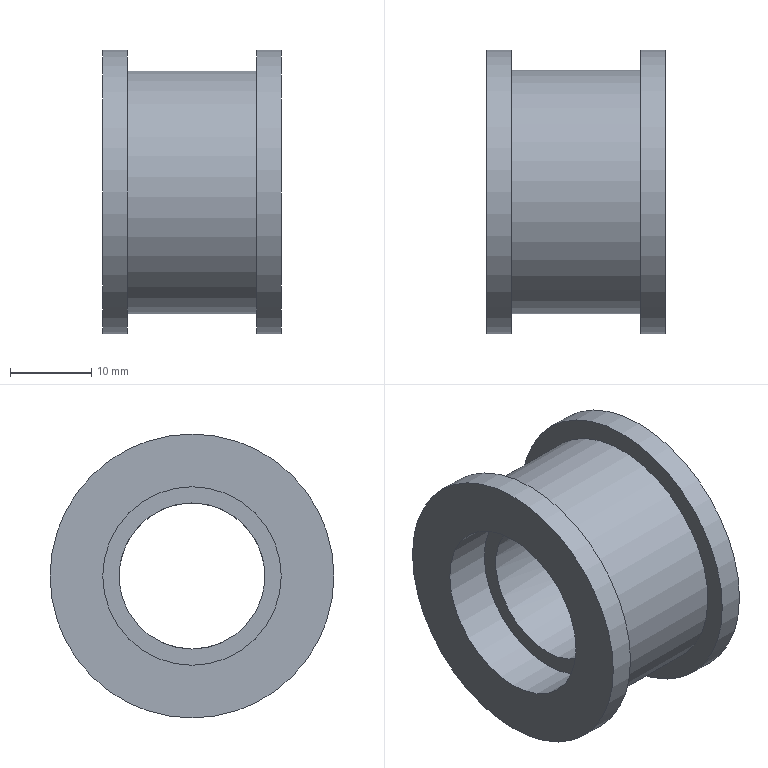Part | NX | 1 solid | 12 faces | box 22 x 35 x 35 mm | volume 9976 mm3 | plane 6 | cylinder 6 | commonest cylinder face diameters 22 x2 35 x2 18 x1 30 x1
STEP:
#1=CARTESIAN_POINT('',(-11.,0.,-17.5));
#2=VERTEX_POINT('',#1);
#3=CARTESIAN_POINT('',(-11.,0.,0.));
#4=DIRECTION('',(1.,0.,0.));
#5=DIRECTION('',(0.,0.,-1.));
#6=AXIS2_PLACEMENT_3D('',#3,#4,#5);
#7=CIRCLE('',#6,17.5);
#8=EDGE_CURVE('',#2,#2,#7,.T.);
#9=ORIENTED_EDGE('',*,*,#8,.F.);
#10=EDGE_LOOP('',(#9));
#11=FACE_BOUND('',#10,.T.);
#12=CARTESIAN_POINT('',(-11.,0.,-11.));
#13=VERTEX_POINT('',#12);
#14=CARTESIAN_POINT('',(-11.,0.,0.));
#15=DIRECTION('',(1.,0.,0.));
#16=DIRECTION('',(0.,0.,-1.));
#17=AXIS2_PLACEMENT_3D('',#14,#15,#16);
#18=CIRCLE('',#17,11.);
#19=EDGE_CURVE('',#13,#13,#18,.T.);
#20=ORIENTED_EDGE('',*,*,#19,.T.);
#21=EDGE_LOOP('',(#20));
#22=FACE_BOUND('',#21,.T.);
#23=CARTESIAN_POINT('',(-11.,0.,0.));
#24=DIRECTION('',(1.,0.,0.));
#25=DIRECTION('',(0.,0.,-1.));
#26=AXIS2_PLACEMENT_3D('',#23,#24,#25);
#27=PLANE('',#26);
#28=ADVANCED_FACE('',(#11,#22),#27,.F.);
#29=ORIENTED_EDGE('',*,*,#8,.T.);
#30=EDGE_LOOP('',(#29));
#31=FACE_BOUND('',#30,.T.);
#32=CARTESIAN_POINT('',(-8.,0.,-17.5));
#33=VERTEX_POINT('',#32);
#34=CARTESIAN_POINT('',(-8.,0.,0.));
#35=DIRECTION('',(1.,0.,0.));
#36=DIRECTION('',(0.,0.,-1.));
#37=AXIS2_PLACEMENT_3D('',#34,#35,#36);
#38=CIRCLE('',#37,17.5);
#39=EDGE_CURVE('',#33,#33,#38,.T.);
#40=ORIENTED_EDGE('',*,*,#39,.F.);
#41=EDGE_LOOP('',(#40));
#42=FACE_BOUND('',#41,.T.);
#43=CARTESIAN_POINT('',(11.,0.,0.));
#44=DIRECTION('',(-1.,0.,0.));
#45=DIRECTION('',(0.,0.,1.));
#46=AXIS2_PLACEMENT_3D('',#43,#44,#45);
#47=CYLINDRICAL_SURFACE('',#46,17.5);
#48=ADVANCED_FACE('',(#31,#42),#47,.T.);
#49=CARTESIAN_POINT('',(-8.,0.,-15.));
#50=VERTEX_POINT('',#49);
#51=CARTESIAN_POINT('',(-8.,0.,0.));
#52=DIRECTION('',(1.,0.,0.));
#53=DIRECTION('',(0.,0.,-1.));
#54=AXIS2_PLACEMENT_3D('',#51,#52,#53);
#55=CIRCLE('',#54,15.);
#56=EDGE_CURVE('',#50,#50,#55,.T.);
#57=ORIENTED_EDGE('',*,*,#56,.F.);
#58=EDGE_LOOP('',(#57));
#59=FACE_BOUND('',#58,.T.);
#60=ORIENTED_EDGE('',*,*,#39,.T.);
#61=EDGE_LOOP('',(#60));
#62=FACE_BOUND('',#61,.T.);
#63=CARTESIAN_POINT('',(-8.,0.,0.));
#64=DIRECTION('',(1.,0.,0.));
#65=DIRECTION('',(0.,0.,-1.));
#66=AXIS2_PLACEMENT_3D('',#63,#64,#65);
#67=PLANE('',#66);
#68=ADVANCED_FACE('',(#59,#62),#67,.T.);
#69=CARTESIAN_POINT('',(8.,0.,-15.));
#70=VERTEX_POINT('',#69);
#71=CARTESIAN_POINT('',(8.,0.,0.));
#72=DIRECTION('',(1.,0.,0.));
#73=DIRECTION('',(0.,0.,-1.));
#74=AXIS2_PLACEMENT_3D('',#71,#72,#73);
#75=CIRCLE('',#74,15.);
#76=EDGE_CURVE('',#70,#70,#75,.T.);
#77=ORIENTED_EDGE('',*,*,#76,.T.);
#78=EDGE_LOOP('',(#77));
#79=FACE_BOUND('',#78,.T.);
#80=CARTESIAN_POINT('',(8.,0.,-17.5));
#81=VERTEX_POINT('',#80);
#82=CARTESIAN_POINT('',(8.,0.,0.));
#83=DIRECTION('',(1.,0.,0.));
#84=DIRECTION('',(0.,0.,-1.));
#85=AXIS2_PLACEMENT_3D('',#82,#83,#84);
#86=CIRCLE('',#85,17.5);
#87=EDGE_CURVE('',#81,#81,#86,.T.);
#88=ORIENTED_EDGE('',*,*,#87,.F.);
#89=EDGE_LOOP('',(#88));
#90=FACE_BOUND('',#89,.T.);
#91=CARTESIAN_POINT('',(8.,0.,0.));
#92=DIRECTION('',(1.,0.,0.));
#93=DIRECTION('',(0.,0.,-1.));
#94=AXIS2_PLACEMENT_3D('',#91,#92,#93);
#95=PLANE('',#94);
#96=ADVANCED_FACE('',(#79,#90),#95,.F.);
#97=ORIENTED_EDGE('',*,*,#56,.T.);
#98=EDGE_LOOP('',(#97));
#99=FACE_BOUND('',#98,.T.);
#100=ORIENTED_EDGE('',*,*,#76,.F.);
#101=EDGE_LOOP('',(#100));
#102=FACE_BOUND('',#101,.T.);
#103=CARTESIAN_POINT('',(-8.,0.,0.));
#104=DIRECTION('',(1.,0.,0.));
#105=DIRECTION('',(0.,0.,-1.));
#106=AXIS2_PLACEMENT_3D('',#103,#104,#105);
#107=CYLINDRICAL_SURFACE('',#106,15.);
#108=ADVANCED_FACE('',(#99,#102),#107,.T.);
#109=CARTESIAN_POINT('',(11.,0.,-11.));
#110=VERTEX_POINT('',#109);
#111=CARTESIAN_POINT('',(11.,0.,0.));
#112=DIRECTION('',(1.,0.,0.));
#113=DIRECTION('',(0.,0.,-1.));
#114=AXIS2_PLACEMENT_3D('',#111,#112,#113);
#115=CIRCLE('',#114,11.);
#116=EDGE_CURVE('',#110,#110,#115,.T.);
#117=ORIENTED_EDGE('',*,*,#116,.F.);
#118=EDGE_LOOP('',(#117));
#119=FACE_BOUND('',#118,.T.);
#120=CARTESIAN_POINT('',(11.,0.,-17.5));
#121=VERTEX_POINT('',#120);
#122=CARTESIAN_POINT('',(11.,0.,0.));
#123=DIRECTION('',(1.,0.,0.));
#124=DIRECTION('',(0.,0.,-1.));
#125=AXIS2_PLACEMENT_3D('',#122,#123,#124);
#126=CIRCLE('',#125,17.5);
#127=EDGE_CURVE('',#121,#121,#126,.T.);
#128=ORIENTED_EDGE('',*,*,#127,.T.);
#129=EDGE_LOOP('',(#128));
#130=FACE_BOUND('',#129,.T.);
#131=CARTESIAN_POINT('',(11.,0.,0.));
#132=DIRECTION('',(1.,0.,0.));
#133=DIRECTION('',(0.,0.,-1.));
#134=AXIS2_PLACEMENT_3D('',#131,#132,#133);
#135=PLANE('',#134);
#136=ADVANCED_FACE('',(#119,#130),#135,.T.);
#137=ORIENTED_EDGE('',*,*,#87,.T.);
#138=EDGE_LOOP('',(#137));
#139=FACE_BOUND('',#138,.T.);
#140=ORIENTED_EDGE('',*,*,#127,.F.);
#141=EDGE_LOOP('',(#140));
#142=FACE_BOUND('',#141,.T.);
#143=CARTESIAN_POINT('',(11.,0.,0.));
#144=DIRECTION('',(-1.,0.,0.));
#145=DIRECTION('',(0.,0.,1.));
#146=AXIS2_PLACEMENT_3D('',#143,#144,#145);
#147=CYLINDRICAL_SURFACE('',#146,17.5);
#148=ADVANCED_FACE('',(#139,#142),#147,.T.);
#149=CARTESIAN_POINT('',(5.,0.,-11.));
#150=VERTEX_POINT('',#149);
#151=CARTESIAN_POINT('',(5.,0.,0.));
#152=DIRECTION('',(1.,0.,0.));
#153=DIRECTION('',(0.,0.,-1.));
#154=AXIS2_PLACEMENT_3D('',#151,#152,#153);
#155=CIRCLE('',#154,11.);
#156=EDGE_CURVE('',#150,#150,#155,.T.);
#157=ORIENTED_EDGE('',*,*,#156,.F.);
#158=EDGE_LOOP('',(#157));
#159=FACE_BOUND('',#158,.T.);
#160=ORIENTED_EDGE('',*,*,#116,.T.);
#161=EDGE_LOOP('',(#160));
#162=FACE_BOUND('',#161,.T.);
#163=CARTESIAN_POINT('',(5.,0.,0.));
#164=DIRECTION('',(1.,0.,0.));
#165=DIRECTION('',(0.,0.,-1.));
#166=AXIS2_PLACEMENT_3D('',#163,#164,#165);
#167=CYLINDRICAL_SURFACE('',#166,11.);
#168=ADVANCED_FACE('',(#159,#162),#167,.F.);
#169=CARTESIAN_POINT('',(5.,0.,-9.));
#170=VERTEX_POINT('',#169);
#171=CARTESIAN_POINT('',(5.,0.,0.));
#172=DIRECTION('',(1.,0.,0.));
#173=DIRECTION('',(0.,0.,-1.));
#174=AXIS2_PLACEMENT_3D('',#171,#172,#173);
#175=CIRCLE('',#174,9.);
#176=EDGE_CURVE('',#170,#170,#175,.T.);
#177=ORIENTED_EDGE('',*,*,#176,.F.);
#178=EDGE_LOOP('',(#177));
#179=FACE_BOUND('',#178,.T.);
#180=ORIENTED_EDGE('',*,*,#156,.T.);
#181=EDGE_LOOP('',(#180));
#182=FACE_BOUND('',#181,.T.);
#183=CARTESIAN_POINT('',(5.,0.,0.));
#184=DIRECTION('',(1.,0.,0.));
#185=DIRECTION('',(0.,0.,-1.));
#186=AXIS2_PLACEMENT_3D('',#183,#184,#185);
#187=PLANE('',#186);
#188=ADVANCED_FACE('',(#179,#182),#187,.T.);
#189=CARTESIAN_POINT('',(-5.,0.,-11.));
#190=VERTEX_POINT('',#189);
#191=CARTESIAN_POINT('',(-5.,0.,0.));
#192=DIRECTION('',(1.,0.,0.));
#193=DIRECTION('',(0.,0.,-1.));
#194=AXIS2_PLACEMENT_3D('',#191,#192,#193);
#195=CIRCLE('',#194,11.);
#196=EDGE_CURVE('',#190,#190,#195,.T.);
#197=ORIENTED_EDGE('',*,*,#196,.T.);
#198=EDGE_LOOP('',(#197));
#199=FACE_BOUND('',#198,.T.);
#200=ORIENTED_EDGE('',*,*,#19,.F.);
#201=EDGE_LOOP('',(#200));
#202=FACE_BOUND('',#201,.T.);
#203=CARTESIAN_POINT('',(-5.,0.,0.));
#204=DIRECTION('',(-1.,0.,0.));
#205=DIRECTION('',(0.,0.,1.));
#206=AXIS2_PLACEMENT_3D('',#203,#204,#205);
#207=CYLINDRICAL_SURFACE('',#206,11.);
#208=ADVANCED_FACE('',(#199,#202),#207,.F.);
#209=CARTESIAN_POINT('',(-5.,0.,9.));
#210=VERTEX_POINT('',#209);
#211=CARTESIAN_POINT('',(-5.,0.,0.));
#212=DIRECTION('',(-1.,0.,0.));
#213=DIRECTION('',(0.,0.,1.));
#214=AXIS2_PLACEMENT_3D('',#211,#212,#213);
#215=CIRCLE('',#214,9.);
#216=EDGE_CURVE('',#210,#210,#215,.T.);
#217=ORIENTED_EDGE('',*,*,#216,.F.);
#218=EDGE_LOOP('',(#217));
#219=FACE_BOUND('',#218,.T.);
#220=ORIENTED_EDGE('',*,*,#196,.F.);
#221=EDGE_LOOP('',(#220));
#222=FACE_BOUND('',#221,.T.);
#223=CARTESIAN_POINT('',(-5.,0.,0.));
#224=DIRECTION('',(-1.,0.,0.));
#225=DIRECTION('',(0.,0.,-1.));
#226=AXIS2_PLACEMENT_3D('',#223,#224,#225);
#227=PLANE('',#226);
#228=ADVANCED_FACE('',(#219,#222),#227,.T.);
#229=ORIENTED_EDGE('',*,*,#216,.T.);
#230=EDGE_LOOP('',(#229));
#231=FACE_BOUND('',#230,.T.);
#232=ORIENTED_EDGE('',*,*,#176,.T.);
#233=EDGE_LOOP('',(#232));
#234=FACE_BOUND('',#233,.T.);
#235=CARTESIAN_POINT('',(-11.,0.,0.));
#236=DIRECTION('',(1.,0.,0.));
#237=DIRECTION('',(0.,0.,-1.));
#238=AXIS2_PLACEMENT_3D('',#235,#236,#237);
#239=CYLINDRICAL_SURFACE('',#238,9.);
#240=ADVANCED_FACE('',(#231,#234),#239,.F.);
#241=CLOSED_SHELL('',(#28,#48,#68,#96,#108,#136,#148,#168,#188,#208,#228,#240));
#242=MANIFOLD_SOLID_BREP('',#241);
#243=(LENGTH_UNIT()NAMED_UNIT(*)SI_UNIT(.MILLI.,.METRE.));
#244=UNCERTAINTY_MEASURE_WITH_UNIT(LENGTH_MEASURE(0.00001),#243,'','');
#245=(NAMED_UNIT(*)PLANE_ANGLE_UNIT()SI_UNIT($,.RADIAN.));
#246=(NAMED_UNIT(*)SI_UNIT($,.STERADIAN.)SOLID_ANGLE_UNIT());
#247=(GEOMETRIC_REPRESENTATION_CONTEXT(3)GLOBAL_UNCERTAINTY_ASSIGNED_CONTEXT((#244))GLOBAL_UNIT_ASSIGNED_CONTEXT((#243,#245,#246))REPRESENTATION_CONTEXT('',''));
#248=ADVANCED_BREP_SHAPE_REPRESENTATION('',(#242),#247);